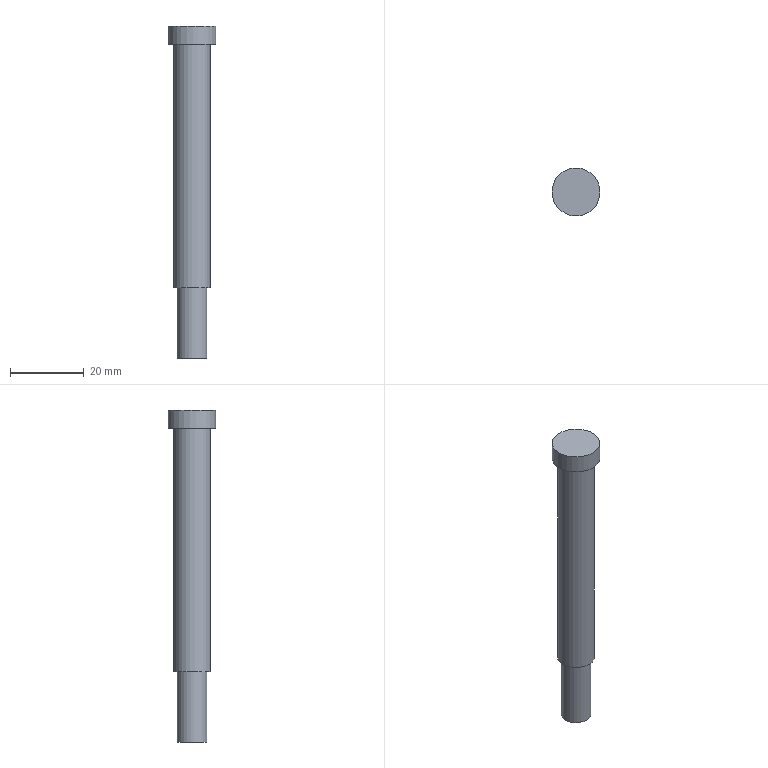Part | NX | features solid 2 | 1 solid | 7 faces | box 13 x 13 x 90 mm | volume 6826 mm3 | plane 4 | cylinder 3 | commonest cylinder face diameters 8.1 x1 10 x1 13 x1
STEP:
#1=CARTESIAN_POINT('',(523.579,-186.178,32.));
#2=VERTEX_POINT('',#1);
#3=CARTESIAN_POINT('',(520.365,-190.008,32.));
#4=DIRECTION('',(0.,0.,-1.));
#5=DIRECTION('',(0.6428,0.766,0.));
#6=AXIS2_PLACEMENT_3D('',#3,#4,#5);
#7=CIRCLE('',#6,5.);
#8=EDGE_CURVE('',#2,#2,#7,.T.);
#9=ORIENTED_EDGE('',*,*,#8,.F.);
#10=EDGE_LOOP('',(#9));
#11=FACE_BOUND('',#10,.T.);
#12=CARTESIAN_POINT('',(523.579,-186.178,98.));
#13=VERTEX_POINT('',#12);
#14=CARTESIAN_POINT('',(520.365,-190.008,98.));
#15=DIRECTION('',(0.,0.,-1.));
#16=DIRECTION('',(0.6428,0.766,0.));
#17=AXIS2_PLACEMENT_3D('',#14,#15,#16);
#18=CIRCLE('',#17,5.);
#19=EDGE_CURVE('',#13,#13,#18,.T.);
#20=ORIENTED_EDGE('',*,*,#19,.T.);
#21=EDGE_LOOP('',(#20));
#22=FACE_BOUND('',#21,.T.);
#23=CARTESIAN_POINT('',(520.365,-190.008,103.));
#24=DIRECTION('',(0.,0.,-1.));
#25=DIRECTION('',(-0.6428,-0.766,0.));
#26=AXIS2_PLACEMENT_3D('',#23,#24,#25);
#27=CYLINDRICAL_SURFACE('',#26,5.);
#28=ADVANCED_FACE('',(#11,#22),#27,.T.);
#29=CARTESIAN_POINT('',(522.968,-186.905,32.));
#30=VERTEX_POINT('',#29);
#31=CARTESIAN_POINT('',(520.365,-190.008,32.));
#32=DIRECTION('',(0.,0.,-1.));
#33=DIRECTION('',(0.6428,0.766,0.));
#34=AXIS2_PLACEMENT_3D('',#31,#32,#33);
#35=CIRCLE('',#34,4.05);
#36=EDGE_CURVE('',#30,#30,#35,.T.);
#37=ORIENTED_EDGE('',*,*,#36,.F.);
#38=EDGE_LOOP('',(#37));
#39=FACE_BOUND('',#38,.T.);
#40=ORIENTED_EDGE('',*,*,#8,.T.);
#41=EDGE_LOOP('',(#40));
#42=FACE_BOUND('',#41,.T.);
#43=CARTESIAN_POINT('',(520.365,-190.008,32.));
#44=DIRECTION('',(0.,0.,1.));
#45=DIRECTION('',(0.6428,0.766,0.));
#46=AXIS2_PLACEMENT_3D('',#43,#44,#45);
#47=PLANE('',#46);
#48=ADVANCED_FACE('',(#39,#42),#47,.F.);
#49=CARTESIAN_POINT('',(524.543,-185.029,98.));
#50=VERTEX_POINT('',#49);
#51=CARTESIAN_POINT('',(520.365,-190.008,98.));
#52=DIRECTION('',(0.,0.,-1.));
#53=DIRECTION('',(0.6428,0.766,0.));
#54=AXIS2_PLACEMENT_3D('',#51,#52,#53);
#55=CIRCLE('',#54,6.5);
#56=EDGE_CURVE('',#50,#50,#55,.T.);
#57=ORIENTED_EDGE('',*,*,#56,.T.);
#58=EDGE_LOOP('',(#57));
#59=FACE_BOUND('',#58,.T.);
#60=ORIENTED_EDGE('',*,*,#19,.F.);
#61=EDGE_LOOP('',(#60));
#62=FACE_BOUND('',#61,.T.);
#63=CARTESIAN_POINT('',(520.365,-190.008,98.));
#64=DIRECTION('',(0.,0.,1.));
#65=DIRECTION('',(0.6428,0.766,0.));
#66=AXIS2_PLACEMENT_3D('',#63,#64,#65);
#67=PLANE('',#66);
#68=ADVANCED_FACE('',(#59,#62),#67,.F.);
#69=ORIENTED_EDGE('',*,*,#56,.F.);
#70=EDGE_LOOP('',(#69));
#71=FACE_BOUND('',#70,.T.);
#72=CARTESIAN_POINT('',(524.543,-185.029,103.));
#73=VERTEX_POINT('',#72);
#74=CARTESIAN_POINT('',(520.365,-190.008,103.));
#75=DIRECTION('',(0.,0.,-1.));
#76=DIRECTION('',(0.6428,0.766,0.));
#77=AXIS2_PLACEMENT_3D('',#74,#75,#76);
#78=CIRCLE('',#77,6.5);
#79=EDGE_CURVE('',#73,#73,#78,.T.);
#80=ORIENTED_EDGE('',*,*,#79,.T.);
#81=EDGE_LOOP('',(#80));
#82=FACE_BOUND('',#81,.T.);
#83=CARTESIAN_POINT('',(520.365,-190.008,98.));
#84=DIRECTION('',(0.,0.,1.));
#85=DIRECTION('',(0.6428,0.766,0.));
#86=AXIS2_PLACEMENT_3D('',#83,#84,#85);
#87=CYLINDRICAL_SURFACE('',#86,6.5);
#88=ADVANCED_FACE('',(#71,#82),#87,.T.);
#89=ORIENTED_EDGE('',*,*,#79,.F.);
#90=EDGE_LOOP('',(#89));
#91=FACE_BOUND('',#90,.T.);
#92=CARTESIAN_POINT('',(520.365,-190.008,103.));
#93=DIRECTION('',(0.,0.,1.));
#94=DIRECTION('',(0.6428,0.766,0.));
#95=AXIS2_PLACEMENT_3D('',#92,#93,#94);
#96=PLANE('',#95);
#97=ADVANCED_FACE('',(#91),#96,.T.);
#98=CARTESIAN_POINT('',(522.968,-186.905,13.));
#99=VERTEX_POINT('',#98);
#100=CARTESIAN_POINT('',(520.365,-190.008,13.));
#101=DIRECTION('',(0.,0.,-1.));
#102=DIRECTION('',(0.6428,0.766,0.));
#103=AXIS2_PLACEMENT_3D('',#100,#101,#102);
#104=CIRCLE('',#103,4.05);
#105=EDGE_CURVE('',#99,#99,#104,.T.);
#106=ORIENTED_EDGE('',*,*,#105,.F.);
#107=EDGE_LOOP('',(#106));
#108=FACE_BOUND('',#107,.T.);
#109=ORIENTED_EDGE('',*,*,#36,.T.);
#110=EDGE_LOOP('',(#109));
#111=FACE_BOUND('',#110,.T.);
#112=CARTESIAN_POINT('',(520.365,-190.008,13.));
#113=DIRECTION('',(0.,0.,1.));
#114=DIRECTION('',(0.6428,0.766,0.));
#115=AXIS2_PLACEMENT_3D('',#112,#113,#114);
#116=CYLINDRICAL_SURFACE('',#115,4.05);
#117=ADVANCED_FACE('',(#108,#111),#116,.T.);
#118=ORIENTED_EDGE('',*,*,#105,.T.);
#119=EDGE_LOOP('',(#118));
#120=FACE_BOUND('',#119,.T.);
#121=CARTESIAN_POINT('',(520.365,-190.008,13.));
#122=DIRECTION('',(0.,0.,1.));
#123=DIRECTION('',(0.6428,0.766,0.));
#124=AXIS2_PLACEMENT_3D('',#121,#122,#123);
#125=PLANE('',#124);
#126=ADVANCED_FACE('',(#120),#125,.F.);
#127=CLOSED_SHELL('',(#28,#48,#68,#88,#97,#117,#126));
#128=MANIFOLD_SOLID_BREP('',#127);
#129=(LENGTH_UNIT()NAMED_UNIT(*)SI_UNIT(.MILLI.,.METRE.));
#130=UNCERTAINTY_MEASURE_WITH_UNIT(LENGTH_MEASURE(0.00001),#129,'','');
#131=(NAMED_UNIT(*)PLANE_ANGLE_UNIT()SI_UNIT($,.RADIAN.));
#132=(NAMED_UNIT(*)SI_UNIT($,.STERADIAN.)SOLID_ANGLE_UNIT());
#133=(GEOMETRIC_REPRESENTATION_CONTEXT(3)GLOBAL_UNCERTAINTY_ASSIGNED_CONTEXT((#130))GLOBAL_UNIT_ASSIGNED_CONTEXT((#129,#131,#132))REPRESENTATION_CONTEXT('',''));
#134=ADVANCED_BREP_SHAPE_REPRESENTATION('',(#128),#133);